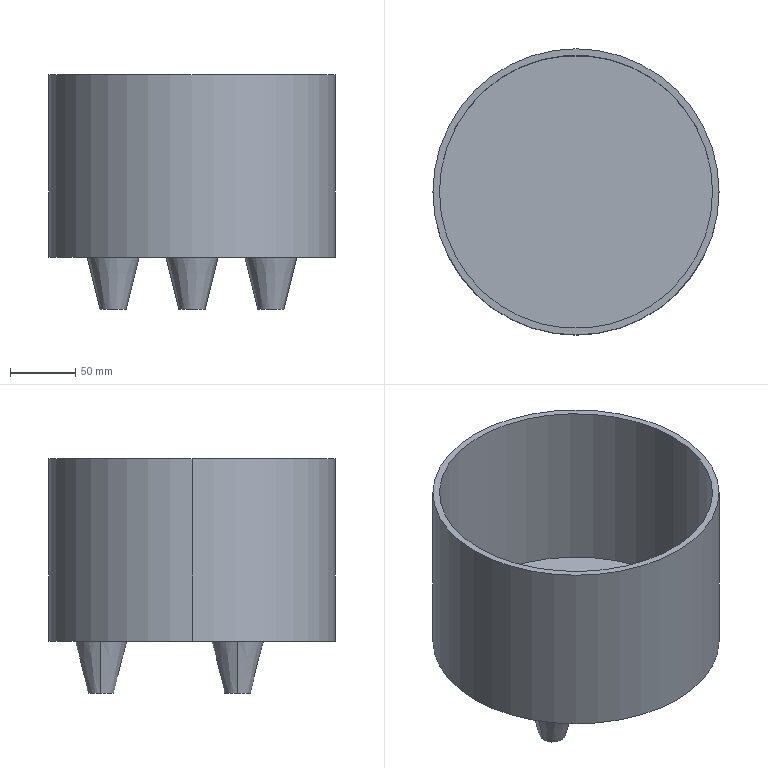Part | STEP file | 333_4 | 1 solid | 16 faces | box 220 x 220 x 180 mm | volume 733955 mm3 | cone 6 | plane 6 | cylinder 4 | commonest cylinder face diameters 210 x2 220 x2
STEP:
#1=CARTESIAN_POINT('',(0.,0.,0.));
#2=DIRECTION('',(0.,0.,1.));
#3=DIRECTION('',(1.,0.,0.));
#4=AXIS2_PLACEMENT_3D('',#1,#2,#3);
#5=CARTESIAN_POINT('',(-110.,0.,40.));
#6=VERTEX_POINT('',#5);
#7=CARTESIAN_POINT('',(110.,0.,40.));
#8=VERTEX_POINT('',#7);
#9=CARTESIAN_POINT('',(0.,0.,40.));
#10=DIRECTION('',(0.,0.,-1.));
#11=DIRECTION('',(-1.,0.,0.));
#12=AXIS2_PLACEMENT_3D('',#9,#10,#11);
#13=CIRCLE('',#12,110.);
#14=CARTESIAN_POINT('',(0.,0.,-30.));
#15=DIRECTION('',(0.,0.,-1.));
#16=DIRECTION('',(-1.,0.,0.));
#17=AXIS2_PLACEMENT_3D('',#14,#15,#16);
#18=CYLINDRICAL_SURFACE('',#17,110.);
#19=CARTESIAN_POINT('',(0.,-70.));
#20=DIRECTION('',(1.,0.));
#21=VECTOR('',#20,1.);
#22=LINE('',#19,#21);
#23=(GEOMETRIC_REPRESENTATION_CONTEXT(2)PARAMETRIC_REPRESENTATION_CONTEXT()REPRESENTATION_CONTEXT('',''));
#24=DEFINITIONAL_REPRESENTATION('',(#22),#23);
#25=PCURVE('',#18,#24);
#26=CARTESIAN_POINT('',(0.,0.,40.));
#27=DIRECTION('',(0.,0.,-1.));
#28=DIRECTION('',(-1.,0.,0.));
#29=AXIS2_PLACEMENT_3D('',#26,#27,#28);
#30=PLANE('',#29);
#31=CARTESIAN_POINT('',(0.,0.));
#32=DIRECTION('',(1.,0.));
#33=AXIS2_PLACEMENT_2D('',#31,#32);
#34=CIRCLE('',#33,110.);
#35=(GEOMETRIC_REPRESENTATION_CONTEXT(2)PARAMETRIC_REPRESENTATION_CONTEXT()REPRESENTATION_CONTEXT('',''));
#36=DEFINITIONAL_REPRESENTATION('',(#34),#35);
#37=PCURVE('',#30,#36);
#38=SURFACE_CURVE('',#13,(#25,#37),.PCURVE_S1.);
#39=EDGE_CURVE('',#6,#8,#38,.T.);
#40=ORIENTED_EDGE('',*,*,#39,.T.);
#41=CARTESIAN_POINT('',(110.,0.,-100.));
#42=VERTEX_POINT('',#41);
#43=CARTESIAN_POINT('',(110.,0.,-30.));
#44=DIRECTION('',(0.,0.,-1.));
#45=VECTOR('',#44,1.);
#46=LINE('',#43,#45);
#47=CARTESIAN_POINT('',(3.142,0.));
#48=DIRECTION('',(0.,1.));
#49=VECTOR('',#48,1.);
#50=LINE('',#47,#49);
#51=(GEOMETRIC_REPRESENTATION_CONTEXT(2)PARAMETRIC_REPRESENTATION_CONTEXT()REPRESENTATION_CONTEXT('',''));
#52=DEFINITIONAL_REPRESENTATION('',(#50),#51);
#53=PCURVE('',#18,#52);
#54=CARTESIAN_POINT('',(0.,0.,-30.));
#55=DIRECTION('',(0.,0.,-1.));
#56=DIRECTION('',(-1.,0.,0.));
#57=AXIS2_PLACEMENT_3D('',#54,#55,#56);
#58=CYLINDRICAL_SURFACE('',#57,110.);
#59=CARTESIAN_POINT('',(3.142,0.));
#60=DIRECTION('',(0.,1.));
#61=VECTOR('',#60,1.);
#62=LINE('',#59,#61);
#63=(GEOMETRIC_REPRESENTATION_CONTEXT(2)PARAMETRIC_REPRESENTATION_CONTEXT()REPRESENTATION_CONTEXT('',''));
#64=DEFINITIONAL_REPRESENTATION('',(#62),#63);
#65=PCURVE('',#58,#64);
#66=SURFACE_CURVE('',#46,(#53,#65),.PCURVE_S1.);
#67=EDGE_CURVE('',#8,#42,#66,.T.);
#68=ORIENTED_EDGE('',*,*,#67,.T.);
#69=CARTESIAN_POINT('',(-110.,0.,-100.));
#70=VERTEX_POINT('',#69);
#71=CARTESIAN_POINT('',(0.,0.,-100.));
#72=DIRECTION('',(0.,0.,1.));
#73=DIRECTION('',(-1.,0.,0.));
#74=AXIS2_PLACEMENT_3D('',#71,#72,#73);
#75=CIRCLE('',#74,110.);
#76=CARTESIAN_POINT('',(6.283,70.));
#77=DIRECTION('',(-1.,0.));
#78=VECTOR('',#77,1.);
#79=LINE('',#76,#78);
#80=(GEOMETRIC_REPRESENTATION_CONTEXT(2)PARAMETRIC_REPRESENTATION_CONTEXT()REPRESENTATION_CONTEXT('',''));
#81=DEFINITIONAL_REPRESENTATION('',(#79),#80);
#82=PCURVE('',#18,#81);
#83=CARTESIAN_POINT('',(-110.,0.,-100.));
#84=DIRECTION('',(0.,0.,-1.));
#85=DIRECTION('',(-1.,0.,0.));
#86=AXIS2_PLACEMENT_3D('',#83,#84,#85);
#87=PLANE('',#86);
#88=CARTESIAN_POINT('',(0.,0.));
#89=CARTESIAN_POINT('',(0.,-190.526));
#90=CARTESIAN_POINT('',(-165.,-95.263));
#91=CARTESIAN_POINT('',(-330.,0.));
#92=CARTESIAN_POINT('',(-165.,95.263));
#93=CARTESIAN_POINT('',(0.,190.526));
#94=CARTESIAN_POINT('',(0.,0.));
#95=(BOUNDED_CURVE()B_SPLINE_CURVE(2,(#88,#89,#90,#91,#92,#93,#94),.UNSPECIFIED.,.T.,.F.)B_SPLINE_CURVE_WITH_KNOTS((1,2,2,2,2,1),(-2.094,0.,2.094,4.189,6.283,8.378),.UNSPECIFIED.)CURVE()GEOMETRIC_REPRESENTATION_ITEM()RATIONAL_B_SPLINE_CURVE((1.,0.5,1.,0.5,1.,0.5,1.))REPRESENTATION_ITEM(''));
#96=(GEOMETRIC_REPRESENTATION_CONTEXT(2)PARAMETRIC_REPRESENTATION_CONTEXT()REPRESENTATION_CONTEXT('',''));
#97=DEFINITIONAL_REPRESENTATION('',(#95),#96);
#98=PCURVE('',#87,#97);
#99=SURFACE_CURVE('',#75,(#82,#98),.PCURVE_S1.);
#100=EDGE_CURVE('',#42,#70,#99,.T.);
#101=ORIENTED_EDGE('',*,*,#100,.T.);
#102=CARTESIAN_POINT('',(-110.,0.,-30.));
#103=DIRECTION('',(0.,0.,-1.));
#104=VECTOR('',#103,1.);
#105=LINE('',#102,#104);
#106=CARTESIAN_POINT('',(0.,0.));
#107=DIRECTION('',(0.,1.));
#108=VECTOR('',#107,1.);
#109=LINE('',#106,#108);
#110=(GEOMETRIC_REPRESENTATION_CONTEXT(2)PARAMETRIC_REPRESENTATION_CONTEXT()REPRESENTATION_CONTEXT('',''));
#111=DEFINITIONAL_REPRESENTATION('',(#109),#110);
#112=PCURVE('',#18,#111);
#113=CARTESIAN_POINT('',(6.283,0.));
#114=DIRECTION('',(0.,1.));
#115=VECTOR('',#114,1.);
#116=LINE('',#113,#115);
#117=(GEOMETRIC_REPRESENTATION_CONTEXT(2)PARAMETRIC_REPRESENTATION_CONTEXT()REPRESENTATION_CONTEXT('',''));
#118=DEFINITIONAL_REPRESENTATION('',(#116),#117);
#119=PCURVE('',#58,#118);
#120=SURFACE_CURVE('',#105,(#112,#119),.PCURVE_S1.);
#121=EDGE_CURVE('',#6,#70,#120,.T.);
#122=ORIENTED_EDGE('',*,*,#121,.F.);
#123=EDGE_LOOP('',(#40,#68,#101,#122));
#124=FACE_BOUND('',#123,.T.);
#125=ADVANCED_FACE('',(#124),#18,.T.);
#126=CARTESIAN_POINT('',(-105.,0.,40.));
#127=VERTEX_POINT('',#126);
#128=CARTESIAN_POINT('',(-105.,0.,-95.));
#129=VERTEX_POINT('',#128);
#130=CARTESIAN_POINT('',(-105.,0.,-30.));
#131=DIRECTION('',(0.,0.,-1.));
#132=VECTOR('',#131,1.);
#133=LINE('',#130,#132);
#134=CARTESIAN_POINT('',(0.,0.,-30.));
#135=DIRECTION('',(0.,0.,-1.));
#136=DIRECTION('',(-1.,0.,0.));
#137=AXIS2_PLACEMENT_3D('',#134,#135,#136);
#138=CYLINDRICAL_SURFACE('',#137,105.);
#139=CARTESIAN_POINT('',(6.283,0.));
#140=DIRECTION('',(0.,1.));
#141=VECTOR('',#140,1.);
#142=LINE('',#139,#141);
#143=(GEOMETRIC_REPRESENTATION_CONTEXT(2)PARAMETRIC_REPRESENTATION_CONTEXT()REPRESENTATION_CONTEXT('',''));
#144=DEFINITIONAL_REPRESENTATION('',(#142),#143);
#145=PCURVE('',#138,#144);
#146=CARTESIAN_POINT('',(0.,0.,-30.));
#147=DIRECTION('',(0.,0.,-1.));
#148=DIRECTION('',(-1.,0.,0.));
#149=AXIS2_PLACEMENT_3D('',#146,#147,#148);
#150=CYLINDRICAL_SURFACE('',#149,105.);
#151=CARTESIAN_POINT('',(0.,0.));
#152=DIRECTION('',(0.,1.));
#153=VECTOR('',#152,1.);
#154=LINE('',#151,#153);
#155=(GEOMETRIC_REPRESENTATION_CONTEXT(2)PARAMETRIC_REPRESENTATION_CONTEXT()REPRESENTATION_CONTEXT('',''));
#156=DEFINITIONAL_REPRESENTATION('',(#154),#155);
#157=PCURVE('',#150,#156);
#158=SURFACE_CURVE('',#133,(#145,#157),.PCURVE_S1.);
#159=EDGE_CURVE('',#127,#129,#158,.T.);
#160=ORIENTED_EDGE('',*,*,#159,.T.);
#161=CARTESIAN_POINT('',(105.,0.,-95.));
#162=VERTEX_POINT('',#161);
#163=CARTESIAN_POINT('',(0.,0.,-95.));
#164=DIRECTION('',(0.,0.,1.));
#165=DIRECTION('',(-1.,0.,0.));
#166=AXIS2_PLACEMENT_3D('',#163,#164,#165);
#167=CIRCLE('',#166,105.);
#168=CARTESIAN_POINT('',(6.283,65.));
#169=DIRECTION('',(-1.,0.));
#170=VECTOR('',#169,1.);
#171=LINE('',#168,#170);
#172=(GEOMETRIC_REPRESENTATION_CONTEXT(2)PARAMETRIC_REPRESENTATION_CONTEXT()REPRESENTATION_CONTEXT('',''));
#173=DEFINITIONAL_REPRESENTATION('',(#171),#172);
#174=PCURVE('',#138,#173);
#175=CARTESIAN_POINT('',(-110.,0.,-95.));
#176=DIRECTION('',(0.,0.,-1.));
#177=DIRECTION('',(-1.,0.,0.));
#178=AXIS2_PLACEMENT_3D('',#175,#176,#177);
#179=PLANE('',#178);
#180=CARTESIAN_POINT('',(-5.,0.));
#181=CARTESIAN_POINT('',(-5.,-181.865));
#182=CARTESIAN_POINT('',(-162.5,-90.933));
#183=CARTESIAN_POINT('',(-320.,0.));
#184=CARTESIAN_POINT('',(-162.5,90.933));
#185=CARTESIAN_POINT('',(-5.,181.865));
#186=CARTESIAN_POINT('',(-5.,0.));
#187=(BOUNDED_CURVE()B_SPLINE_CURVE(2,(#180,#181,#182,#183,#184,#185,#186),.UNSPECIFIED.,.T.,.F.)B_SPLINE_CURVE_WITH_KNOTS((1,2,2,2,2,1),(-2.094,0.,2.094,4.189,6.283,8.378),.UNSPECIFIED.)CURVE()GEOMETRIC_REPRESENTATION_ITEM()RATIONAL_B_SPLINE_CURVE((1.,0.5,1.,0.5,1.,0.5,1.))REPRESENTATION_ITEM(''));
#188=(GEOMETRIC_REPRESENTATION_CONTEXT(2)PARAMETRIC_REPRESENTATION_CONTEXT()REPRESENTATION_CONTEXT('',''));
#189=DEFINITIONAL_REPRESENTATION('',(#187),#188);
#190=PCURVE('',#179,#189);
#191=SURFACE_CURVE('',#167,(#174,#190),.PCURVE_S1.);
#192=EDGE_CURVE('',#129,#162,#191,.T.);
#193=ORIENTED_EDGE('',*,*,#192,.T.);
#194=CARTESIAN_POINT('',(105.,0.,40.));
#195=VERTEX_POINT('',#194);
#196=CARTESIAN_POINT('',(105.,0.,-30.));
#197=DIRECTION('',(0.,0.,-1.));
#198=VECTOR('',#197,1.);
#199=LINE('',#196,#198);
#200=CARTESIAN_POINT('',(3.142,0.));
#201=DIRECTION('',(0.,1.));
#202=VECTOR('',#201,1.);
#203=LINE('',#200,#202);
#204=(GEOMETRIC_REPRESENTATION_CONTEXT(2)PARAMETRIC_REPRESENTATION_CONTEXT()REPRESENTATION_CONTEXT('',''));
#205=DEFINITIONAL_REPRESENTATION('',(#203),#204);
#206=PCURVE('',#138,#205);
#207=CARTESIAN_POINT('',(3.142,0.));
#208=DIRECTION('',(0.,1.));
#209=VECTOR('',#208,1.);
#210=LINE('',#207,#209);
#211=(GEOMETRIC_REPRESENTATION_CONTEXT(2)PARAMETRIC_REPRESENTATION_CONTEXT()REPRESENTATION_CONTEXT('',''));
#212=DEFINITIONAL_REPRESENTATION('',(#210),#211);
#213=PCURVE('',#150,#212);
#214=SURFACE_CURVE('',#199,(#206,#213),.PCURVE_S1.);
#215=EDGE_CURVE('',#195,#162,#214,.T.);
#216=ORIENTED_EDGE('',*,*,#215,.F.);
#217=CARTESIAN_POINT('',(0.,0.,40.));
#218=DIRECTION('',(0.,0.,1.));
#219=DIRECTION('',(-1.,0.,0.));
#220=AXIS2_PLACEMENT_3D('',#217,#218,#219);
#221=CIRCLE('',#220,105.);
#222=CARTESIAN_POINT('',(6.283,-70.));
#223=DIRECTION('',(-1.,0.));
#224=VECTOR('',#223,1.);
#225=LINE('',#222,#224);
#226=(GEOMETRIC_REPRESENTATION_CONTEXT(2)PARAMETRIC_REPRESENTATION_CONTEXT()REPRESENTATION_CONTEXT('',''));
#227=DEFINITIONAL_REPRESENTATION('',(#225),#226);
#228=PCURVE('',#138,#227);
#229=CARTESIAN_POINT('',(105.,0.));
#230=CARTESIAN_POINT('',(105.,-181.865));
#231=CARTESIAN_POINT('',(-52.5,-90.933));
#232=CARTESIAN_POINT('',(-210.,0.));
#233=CARTESIAN_POINT('',(-52.5,90.933));
#234=CARTESIAN_POINT('',(105.,181.865));
#235=CARTESIAN_POINT('',(105.,0.));
#236=(BOUNDED_CURVE()B_SPLINE_CURVE(2,(#229,#230,#231,#232,#233,#234,#235),.UNSPECIFIED.,.T.,.F.)B_SPLINE_CURVE_WITH_KNOTS((1,2,2,2,2,1),(-2.094,0.,2.094,4.189,6.283,8.378),.UNSPECIFIED.)CURVE()GEOMETRIC_REPRESENTATION_ITEM()RATIONAL_B_SPLINE_CURVE((1.,0.5,1.,0.5,1.,0.5,1.))REPRESENTATION_ITEM(''));
#237=(GEOMETRIC_REPRESENTATION_CONTEXT(2)PARAMETRIC_REPRESENTATION_CONTEXT()REPRESENTATION_CONTEXT('',''));
#238=DEFINITIONAL_REPRESENTATION('',(#236),#237);
#239=PCURVE('',#30,#238);
#240=SURFACE_CURVE('',#221,(#228,#239),.PCURVE_S1.);
#241=EDGE_CURVE('',#127,#195,#240,.T.);
#242=ORIENTED_EDGE('',*,*,#241,.F.);
#243=EDGE_LOOP('',(#160,#193,#216,#242));
#244=FACE_BOUND('',#243,.F.);
#245=ADVANCED_FACE('',(#244),#138,.F.);
#246=CARTESIAN_POINT('',(70.622,-35.,-140.));
#247=VERTEX_POINT('',#246);
#248=CARTESIAN_POINT('',(50.622,-35.,-140.));
#249=VERTEX_POINT('',#248);
#250=CARTESIAN_POINT('',(60.622,-35.,-140.));
#251=DIRECTION('',(0.,0.,1.));
#252=DIRECTION('',(1.,0.,0.));
#253=AXIS2_PLACEMENT_3D('',#250,#251,#252);
#254=CIRCLE('',#253,10.);
#255=CARTESIAN_POINT('',(60.622,-35.,-100.));
#256=DIRECTION('',(0.,0.,1.));
#257=DIRECTION('',(1.,0.,0.));
#258=AXIS2_PLACEMENT_3D('',#255,#256,#257);
#259=CONICAL_SURFACE('',#258,20.,0.245);
#260=CARTESIAN_POINT('',(0.,-40.));
#261=DIRECTION('',(1.,0.));
#262=VECTOR('',#261,1.);
#263=LINE('',#260,#262);
#264=(GEOMETRIC_REPRESENTATION_CONTEXT(2)PARAMETRIC_REPRESENTATION_CONTEXT()REPRESENTATION_CONTEXT('',''));
#265=DEFINITIONAL_REPRESENTATION('',(#263),#264);
#266=PCURVE('',#259,#265);
#267=CARTESIAN_POINT('',(0.,80.,-140.));
#268=DIRECTION('',(0.,0.,-1.));
#269=DIRECTION('',(-1.,0.,0.));
#270=AXIS2_PLACEMENT_3D('',#267,#268,#269);
#271=PLANE('',#270);
#272=CARTESIAN_POINT('',(-70.622,-115.));
#273=CARTESIAN_POINT('',(-70.622,-97.679));
#274=CARTESIAN_POINT('',(-55.622,-106.34));
#275=CARTESIAN_POINT('',(-40.622,-115.));
#276=CARTESIAN_POINT('',(-55.622,-123.66));
#277=CARTESIAN_POINT('',(-70.622,-132.321));
#278=CARTESIAN_POINT('',(-70.622,-115.));
#279=(BOUNDED_CURVE()B_SPLINE_CURVE(2,(#272,#273,#274,#275,#276,#277,#278),.UNSPECIFIED.,.T.,.F.)B_SPLINE_CURVE_WITH_KNOTS((1,2,2,2,2,1),(-2.094,0.,2.094,4.189,6.283,8.378),.UNSPECIFIED.)CURVE()GEOMETRIC_REPRESENTATION_ITEM()RATIONAL_B_SPLINE_CURVE((1.,0.5,1.,0.5,1.,0.5,1.))REPRESENTATION_ITEM(''));
#280=(GEOMETRIC_REPRESENTATION_CONTEXT(2)PARAMETRIC_REPRESENTATION_CONTEXT()REPRESENTATION_CONTEXT('',''));
#281=DEFINITIONAL_REPRESENTATION('',(#279),#280);
#282=PCURVE('',#271,#281);
#283=SURFACE_CURVE('',#254,(#266,#282),.PCURVE_S1.);
#284=EDGE_CURVE('',#247,#249,#283,.T.);
#285=ORIENTED_EDGE('',*,*,#284,.T.);
#286=CARTESIAN_POINT('',(40.622,-35.,-100.));
#287=VERTEX_POINT('',#286);
#288=CARTESIAN_POINT('',(40.622,-35.,-100.));
#289=DIRECTION('',(-0.2425,0.,0.9701));
#290=VECTOR('',#289,1.);
#291=LINE('',#288,#290);
#292=CARTESIAN_POINT('',(3.142,0.));
#293=DIRECTION('',(0.,1.));
#294=VECTOR('',#293,1.);
#295=LINE('',#292,#294);
#296=(GEOMETRIC_REPRESENTATION_CONTEXT(2)PARAMETRIC_REPRESENTATION_CONTEXT()REPRESENTATION_CONTEXT('',''));
#297=DEFINITIONAL_REPRESENTATION('',(#295),#296);
#298=PCURVE('',#259,#297);
#299=CARTESIAN_POINT('',(60.622,-35.,-100.));
#300=DIRECTION('',(0.,0.,1.));
#301=DIRECTION('',(1.,0.,0.));
#302=AXIS2_PLACEMENT_3D('',#299,#300,#301);
#303=CONICAL_SURFACE('',#302,20.,0.245);
#304=CARTESIAN_POINT('',(3.142,0.));
#305=DIRECTION('',(0.,1.));
#306=VECTOR('',#305,1.);
#307=LINE('',#304,#306);
#308=(GEOMETRIC_REPRESENTATION_CONTEXT(2)PARAMETRIC_REPRESENTATION_CONTEXT()REPRESENTATION_CONTEXT('',''));
#309=DEFINITIONAL_REPRESENTATION('',(#307),#308);
#310=PCURVE('',#303,#309);
#311=SURFACE_CURVE('',#291,(#298,#310),.PCURVE_S1.);
#312=EDGE_CURVE('',#249,#287,#311,.T.);
#313=ORIENTED_EDGE('',*,*,#312,.T.);
#314=CARTESIAN_POINT('',(80.622,-35.,-100.));
#315=VERTEX_POINT('',#314);
#316=CARTESIAN_POINT('',(60.622,-35.,-100.));
#317=DIRECTION('',(0.,0.,1.));
#318=DIRECTION('',(1.,0.,0.));
#319=AXIS2_PLACEMENT_3D('',#316,#317,#318);
#320=CIRCLE('',#319,20.);
#321=CARTESIAN_POINT('',(0.,0.));
#322=DIRECTION('',(1.,0.));
#323=VECTOR('',#322,1.);
#324=LINE('',#321,#323);
#325=(GEOMETRIC_REPRESENTATION_CONTEXT(2)PARAMETRIC_REPRESENTATION_CONTEXT()REPRESENTATION_CONTEXT('',''));
#326=DEFINITIONAL_REPRESENTATION('',(#324),#325);
#327=PCURVE('',#259,#326);
#328=CARTESIAN_POINT('',(-190.622,-35.));
#329=CARTESIAN_POINT('',(-190.622,-0.359));
#330=CARTESIAN_POINT('',(-160.622,-17.679));
#331=CARTESIAN_POINT('',(-130.622,-35.));
#332=CARTESIAN_POINT('',(-160.622,-52.321));
#333=CARTESIAN_POINT('',(-190.622,-69.641));
#334=CARTESIAN_POINT('',(-190.622,-35.));
#335=(BOUNDED_CURVE()B_SPLINE_CURVE(2,(#328,#329,#330,#331,#332,#333,#334),.UNSPECIFIED.,.T.,.F.)B_SPLINE_CURVE_WITH_KNOTS((1,2,2,2,2,1),(-2.094,0.,2.094,4.189,6.283,8.378),.UNSPECIFIED.)CURVE()GEOMETRIC_REPRESENTATION_ITEM()RATIONAL_B_SPLINE_CURVE((1.,0.5,1.,0.5,1.,0.5,1.))REPRESENTATION_ITEM(''));
#336=(GEOMETRIC_REPRESENTATION_CONTEXT(2)PARAMETRIC_REPRESENTATION_CONTEXT()REPRESENTATION_CONTEXT('',''));
#337=DEFINITIONAL_REPRESENTATION('',(#335),#336);
#338=PCURVE('',#87,#337);
#339=SURFACE_CURVE('',#320,(#327,#338),.PCURVE_S1.);
#340=EDGE_CURVE('',#315,#287,#339,.T.);
#341=ORIENTED_EDGE('',*,*,#340,.F.);
#342=CARTESIAN_POINT('',(80.622,-35.,-100.));
#343=DIRECTION('',(0.2425,0.,0.9701));
#344=VECTOR('',#343,1.);
#345=LINE('',#342,#344);
#346=CARTESIAN_POINT('',(0.,0.));
#347=DIRECTION('',(0.,1.));
#348=VECTOR('',#347,1.);
#349=LINE('',#346,#348);
#350=(GEOMETRIC_REPRESENTATION_CONTEXT(2)PARAMETRIC_REPRESENTATION_CONTEXT()REPRESENTATION_CONTEXT('',''));
#351=DEFINITIONAL_REPRESENTATION('',(#349),#350);
#352=PCURVE('',#259,#351);
#353=CARTESIAN_POINT('',(6.283,0.));
#354=DIRECTION('',(0.,1.));
#355=VECTOR('',#354,1.);
#356=LINE('',#353,#355);
#357=(GEOMETRIC_REPRESENTATION_CONTEXT(2)PARAMETRIC_REPRESENTATION_CONTEXT()REPRESENTATION_CONTEXT('',''));
#358=DEFINITIONAL_REPRESENTATION('',(#356),#357);
#359=PCURVE('',#303,#358);
#360=SURFACE_CURVE('',#345,(#352,#359),.PCURVE_S1.);
#361=EDGE_CURVE('',#247,#315,#360,.T.);
#362=ORIENTED_EDGE('',*,*,#361,.F.);
#363=EDGE_LOOP('',(#285,#313,#341,#362));
#364=FACE_BOUND('',#363,.T.);
#365=ADVANCED_FACE('',(#364),#259,.T.);
#366=CARTESIAN_POINT('',(-50.622,-35.,-140.));
#367=VERTEX_POINT('',#366);
#368=CARTESIAN_POINT('',(-70.622,-35.,-140.));
#369=VERTEX_POINT('',#368);
#370=CARTESIAN_POINT('',(-60.622,-35.,-140.));
#371=DIRECTION('',(0.,0.,1.));
#372=DIRECTION('',(1.,0.,0.));
#373=AXIS2_PLACEMENT_3D('',#370,#371,#372);
#374=CIRCLE('',#373,10.);
#375=CARTESIAN_POINT('',(-60.622,-35.,-100.));
#376=DIRECTION('',(0.,0.,1.));
#377=DIRECTION('',(1.,0.,0.));
#378=AXIS2_PLACEMENT_3D('',#375,#376,#377);
#379=CONICAL_SURFACE('',#378,20.,0.245);
#380=CARTESIAN_POINT('',(0.,-40.));
#381=DIRECTION('',(1.,0.));
#382=VECTOR('',#381,1.);
#383=LINE('',#380,#382);
#384=(GEOMETRIC_REPRESENTATION_CONTEXT(2)PARAMETRIC_REPRESENTATION_CONTEXT()REPRESENTATION_CONTEXT('',''));
#385=DEFINITIONAL_REPRESENTATION('',(#383),#384);
#386=PCURVE('',#379,#385);
#387=CARTESIAN_POINT('',(0.,80.,-140.));
#388=DIRECTION('',(0.,0.,-1.));
#389=DIRECTION('',(-1.,0.,0.));
#390=AXIS2_PLACEMENT_3D('',#387,#388,#389);
#391=PLANE('',#390);
#392=CARTESIAN_POINT('',(50.622,-115.));
#393=CARTESIAN_POINT('',(50.622,-97.679));
#394=CARTESIAN_POINT('',(65.622,-106.34));
#395=CARTESIAN_POINT('',(80.622,-115.));
#396=CARTESIAN_POINT('',(65.622,-123.66));
#397=CARTESIAN_POINT('',(50.622,-132.321));
#398=CARTESIAN_POINT('',(50.622,-115.));
#399=(BOUNDED_CURVE()B_SPLINE_CURVE(2,(#392,#393,#394,#395,#396,#397,#398),.UNSPECIFIED.,.T.,.F.)B_SPLINE_CURVE_WITH_KNOTS((1,2,2,2,2,1),(-2.094,0.,2.094,4.189,6.283,8.378),.UNSPECIFIED.)CURVE()GEOMETRIC_REPRESENTATION_ITEM()RATIONAL_B_SPLINE_CURVE((1.,0.5,1.,0.5,1.,0.5,1.))REPRESENTATION_ITEM(''));
#400=(GEOMETRIC_REPRESENTATION_CONTEXT(2)PARAMETRIC_REPRESENTATION_CONTEXT()REPRESENTATION_CONTEXT('',''));
#401=DEFINITIONAL_REPRESENTATION('',(#399),#400);
#402=PCURVE('',#391,#401);
#403=SURFACE_CURVE('',#374,(#386,#402),.PCURVE_S1.);
#404=EDGE_CURVE('',#367,#369,#403,.T.);
#405=ORIENTED_EDGE('',*,*,#404,.T.);
#406=CARTESIAN_POINT('',(-80.622,-35.,-100.));
#407=VERTEX_POINT('',#406);
#408=CARTESIAN_POINT('',(-80.622,-35.,-100.));
#409=DIRECTION('',(-0.2425,0.,0.9701));
#410=VECTOR('',#409,1.);
#411=LINE('',#408,#410);
#412=CARTESIAN_POINT('',(3.142,0.));
#413=DIRECTION('',(0.,1.));
#414=VECTOR('',#413,1.);
#415=LINE('',#412,#414);
#416=(GEOMETRIC_REPRESENTATION_CONTEXT(2)PARAMETRIC_REPRESENTATION_CONTEXT()REPRESENTATION_CONTEXT('',''));
#417=DEFINITIONAL_REPRESENTATION('',(#415),#416);
#418=PCURVE('',#379,#417);
#419=CARTESIAN_POINT('',(-60.622,-35.,-100.));
#420=DIRECTION('',(0.,0.,1.));
#421=DIRECTION('',(1.,0.,0.));
#422=AXIS2_PLACEMENT_3D('',#419,#420,#421);
#423=CONICAL_SURFACE('',#422,20.,0.245);
#424=CARTESIAN_POINT('',(3.142,0.));
#425=DIRECTION('',(0.,1.));
#426=VECTOR('',#425,1.);
#427=LINE('',#424,#426);
#428=(GEOMETRIC_REPRESENTATION_CONTEXT(2)PARAMETRIC_REPRESENTATION_CONTEXT()REPRESENTATION_CONTEXT('',''));
#429=DEFINITIONAL_REPRESENTATION('',(#427),#428);
#430=PCURVE('',#423,#429);
#431=SURFACE_CURVE('',#411,(#418,#430),.PCURVE_S1.);
#432=EDGE_CURVE('',#369,#407,#431,.T.);
#433=ORIENTED_EDGE('',*,*,#432,.T.);
#434=CARTESIAN_POINT('',(-40.622,-35.,-100.));
#435=VERTEX_POINT('',#434);
#436=CARTESIAN_POINT('',(-60.622,-35.,-100.));
#437=DIRECTION('',(0.,0.,1.));
#438=DIRECTION('',(1.,0.,0.));
#439=AXIS2_PLACEMENT_3D('',#436,#437,#438);
#440=CIRCLE('',#439,20.);
#441=CARTESIAN_POINT('',(0.,0.));
#442=DIRECTION('',(1.,0.));
#443=VECTOR('',#442,1.);
#444=LINE('',#441,#443);
#445=(GEOMETRIC_REPRESENTATION_CONTEXT(2)PARAMETRIC_REPRESENTATION_CONTEXT()REPRESENTATION_CONTEXT('',''));
#446=DEFINITIONAL_REPRESENTATION('',(#444),#445);
#447=PCURVE('',#379,#446);
#448=CARTESIAN_POINT('',(-69.378,-35.));
#449=CARTESIAN_POINT('',(-69.378,-0.359));
#450=CARTESIAN_POINT('',(-39.378,-17.679));
#451=CARTESIAN_POINT('',(-9.378,-35.));
#452=CARTESIAN_POINT('',(-39.378,-52.321));
#453=CARTESIAN_POINT('',(-69.378,-69.641));
#454=CARTESIAN_POINT('',(-69.378,-35.));
#455=(BOUNDED_CURVE()B_SPLINE_CURVE(2,(#448,#449,#450,#451,#452,#453,#454),.UNSPECIFIED.,.T.,.F.)B_SPLINE_CURVE_WITH_KNOTS((1,2,2,2,2,1),(-2.094,0.,2.094,4.189,6.283,8.378),.UNSPECIFIED.)CURVE()GEOMETRIC_REPRESENTATION_ITEM()RATIONAL_B_SPLINE_CURVE((1.,0.5,1.,0.5,1.,0.5,1.))REPRESENTATION_ITEM(''));
#456=(GEOMETRIC_REPRESENTATION_CONTEXT(2)PARAMETRIC_REPRESENTATION_CONTEXT()REPRESENTATION_CONTEXT('',''));
#457=DEFINITIONAL_REPRESENTATION('',(#455),#456);
#458=PCURVE('',#87,#457);
#459=SURFACE_CURVE('',#440,(#447,#458),.PCURVE_S1.);
#460=EDGE_CURVE('',#435,#407,#459,.T.);
#461=ORIENTED_EDGE('',*,*,#460,.F.);
#462=CARTESIAN_POINT('',(-40.622,-35.,-100.));
#463=DIRECTION('',(0.2425,0.,0.9701));
#464=VECTOR('',#463,1.);
#465=LINE('',#462,#464);
#466=CARTESIAN_POINT('',(0.,0.));
#467=DIRECTION('',(0.,1.));
#468=VECTOR('',#467,1.);
#469=LINE('',#466,#468);
#470=(GEOMETRIC_REPRESENTATION_CONTEXT(2)PARAMETRIC_REPRESENTATION_CONTEXT()REPRESENTATION_CONTEXT('',''));
#471=DEFINITIONAL_REPRESENTATION('',(#469),#470);
#472=PCURVE('',#379,#471);
#473=CARTESIAN_POINT('',(6.283,0.));
#474=DIRECTION('',(0.,1.));
#475=VECTOR('',#474,1.);
#476=LINE('',#473,#475);
#477=(GEOMETRIC_REPRESENTATION_CONTEXT(2)PARAMETRIC_REPRESENTATION_CONTEXT()REPRESENTATION_CONTEXT('',''));
#478=DEFINITIONAL_REPRESENTATION('',(#476),#477);
#479=PCURVE('',#423,#478);
#480=SURFACE_CURVE('',#465,(#472,#479),.PCURVE_S1.);
#481=EDGE_CURVE('',#367,#435,#480,.T.);
#482=ORIENTED_EDGE('',*,*,#481,.F.);
#483=EDGE_LOOP('',(#405,#433,#461,#482));
#484=FACE_BOUND('',#483,.T.);
#485=ADVANCED_FACE('',(#484),#379,.T.);
#486=CARTESIAN_POINT('',(10.,70.,-140.));
#487=VERTEX_POINT('',#486);
#488=CARTESIAN_POINT('',(-10.,70.,-140.));
#489=VERTEX_POINT('',#488);
#490=CARTESIAN_POINT('',(0.,70.,-140.));
#491=DIRECTION('',(0.,0.,1.));
#492=DIRECTION('',(1.,0.,0.));
#493=AXIS2_PLACEMENT_3D('',#490,#491,#492);
#494=CIRCLE('',#493,10.);
#495=CARTESIAN_POINT('',(0.,70.,-100.));
#496=DIRECTION('',(0.,0.,1.));
#497=DIRECTION('',(1.,0.,0.));
#498=AXIS2_PLACEMENT_3D('',#495,#496,#497);
#499=CONICAL_SURFACE('',#498,20.,0.245);
#500=CARTESIAN_POINT('',(0.,-40.));
#501=DIRECTION('',(1.,0.));
#502=VECTOR('',#501,1.);
#503=LINE('',#500,#502);
#504=(GEOMETRIC_REPRESENTATION_CONTEXT(2)PARAMETRIC_REPRESENTATION_CONTEXT()REPRESENTATION_CONTEXT('',''));
#505=DEFINITIONAL_REPRESENTATION('',(#503),#504);
#506=PCURVE('',#499,#505);
#507=CARTESIAN_POINT('',(0.,80.,-140.));
#508=DIRECTION('',(0.,0.,-1.));
#509=DIRECTION('',(-1.,0.,0.));
#510=AXIS2_PLACEMENT_3D('',#507,#508,#509);
#511=PLANE('',#510);
#512=CARTESIAN_POINT('',(-10.,-10.));
#513=CARTESIAN_POINT('',(-10.,7.321));
#514=CARTESIAN_POINT('',(5.,-1.34));
#515=CARTESIAN_POINT('',(20.,-10.));
#516=CARTESIAN_POINT('',(5.,-18.66));
#517=CARTESIAN_POINT('',(-10.,-27.321));
#518=CARTESIAN_POINT('',(-10.,-10.));
#519=(BOUNDED_CURVE()B_SPLINE_CURVE(2,(#512,#513,#514,#515,#516,#517,#518),.UNSPECIFIED.,.T.,.F.)B_SPLINE_CURVE_WITH_KNOTS((1,2,2,2,2,1),(-2.094,0.,2.094,4.189,6.283,8.378),.UNSPECIFIED.)CURVE()GEOMETRIC_REPRESENTATION_ITEM()RATIONAL_B_SPLINE_CURVE((1.,0.5,1.,0.5,1.,0.5,1.))REPRESENTATION_ITEM(''));
#520=(GEOMETRIC_REPRESENTATION_CONTEXT(2)PARAMETRIC_REPRESENTATION_CONTEXT()REPRESENTATION_CONTEXT('',''));
#521=DEFINITIONAL_REPRESENTATION('',(#519),#520);
#522=PCURVE('',#511,#521);
#523=SURFACE_CURVE('',#494,(#506,#522),.PCURVE_S1.);
#524=EDGE_CURVE('',#487,#489,#523,.T.);
#525=ORIENTED_EDGE('',*,*,#524,.T.);
#526=CARTESIAN_POINT('',(-20.,70.,-100.));
#527=VERTEX_POINT('',#526);
#528=CARTESIAN_POINT('',(-20.,70.,-100.));
#529=DIRECTION('',(-0.2425,0.,0.9701));
#530=VECTOR('',#529,1.);
#531=LINE('',#528,#530);
#532=CARTESIAN_POINT('',(3.142,0.));
#533=DIRECTION('',(0.,1.));
#534=VECTOR('',#533,1.);
#535=LINE('',#532,#534);
#536=(GEOMETRIC_REPRESENTATION_CONTEXT(2)PARAMETRIC_REPRESENTATION_CONTEXT()REPRESENTATION_CONTEXT('',''));
#537=DEFINITIONAL_REPRESENTATION('',(#535),#536);
#538=PCURVE('',#499,#537);
#539=CARTESIAN_POINT('',(0.,70.,-100.));
#540=DIRECTION('',(0.,0.,1.));
#541=DIRECTION('',(1.,0.,0.));
#542=AXIS2_PLACEMENT_3D('',#539,#540,#541);
#543=CONICAL_SURFACE('',#542,20.,0.245);
#544=CARTESIAN_POINT('',(3.142,0.));
#545=DIRECTION('',(0.,1.));
#546=VECTOR('',#545,1.);
#547=LINE('',#544,#546);
#548=(GEOMETRIC_REPRESENTATION_CONTEXT(2)PARAMETRIC_REPRESENTATION_CONTEXT()REPRESENTATION_CONTEXT('',''));
#549=DEFINITIONAL_REPRESENTATION('',(#547),#548);
#550=PCURVE('',#543,#549);
#551=SURFACE_CURVE('',#531,(#538,#550),.PCURVE_S1.);
#552=EDGE_CURVE('',#489,#527,#551,.T.);
#553=ORIENTED_EDGE('',*,*,#552,.T.);
#554=CARTESIAN_POINT('',(20.,70.,-100.));
#555=VERTEX_POINT('',#554);
#556=CARTESIAN_POINT('',(0.,70.,-100.));
#557=DIRECTION('',(0.,0.,1.));
#558=DIRECTION('',(1.,0.,0.));
#559=AXIS2_PLACEMENT_3D('',#556,#557,#558);
#560=CIRCLE('',#559,20.);
#561=CARTESIAN_POINT('',(0.,0.));
#562=DIRECTION('',(1.,0.));
#563=VECTOR('',#562,1.);
#564=LINE('',#561,#563);
#565=(GEOMETRIC_REPRESENTATION_CONTEXT(2)PARAMETRIC_REPRESENTATION_CONTEXT()REPRESENTATION_CONTEXT('',''));
#566=DEFINITIONAL_REPRESENTATION('',(#564),#565);
#567=PCURVE('',#499,#566);
#568=CARTESIAN_POINT('',(-130.,70.));
#569=CARTESIAN_POINT('',(-130.,104.641));
#570=CARTESIAN_POINT('',(-100.,87.321));
#571=CARTESIAN_POINT('',(-70.,70.));
#572=CARTESIAN_POINT('',(-100.,52.679));
#573=CARTESIAN_POINT('',(-130.,35.359));
#574=CARTESIAN_POINT('',(-130.,70.));
#575=(BOUNDED_CURVE()B_SPLINE_CURVE(2,(#568,#569,#570,#571,#572,#573,#574),.UNSPECIFIED.,.T.,.F.)B_SPLINE_CURVE_WITH_KNOTS((1,2,2,2,2,1),(-2.094,0.,2.094,4.189,6.283,8.378),.UNSPECIFIED.)CURVE()GEOMETRIC_REPRESENTATION_ITEM()RATIONAL_B_SPLINE_CURVE((1.,0.5,1.,0.5,1.,0.5,1.))REPRESENTATION_ITEM(''));
#576=(GEOMETRIC_REPRESENTATION_CONTEXT(2)PARAMETRIC_REPRESENTATION_CONTEXT()REPRESENTATION_CONTEXT('',''));
#577=DEFINITIONAL_REPRESENTATION('',(#575),#576);
#578=PCURVE('',#87,#577);
#579=SURFACE_CURVE('',#560,(#567,#578),.PCURVE_S1.);
#580=EDGE_CURVE('',#555,#527,#579,.T.);
#581=ORIENTED_EDGE('',*,*,#580,.F.);
#582=CARTESIAN_POINT('',(20.,70.,-100.));
#583=DIRECTION('',(0.2425,0.,0.9701));
#584=VECTOR('',#583,1.);
#585=LINE('',#582,#584);
#586=CARTESIAN_POINT('',(0.,0.));
#587=DIRECTION('',(0.,1.));
#588=VECTOR('',#587,1.);
#589=LINE('',#586,#588);
#590=(GEOMETRIC_REPRESENTATION_CONTEXT(2)PARAMETRIC_REPRESENTATION_CONTEXT()REPRESENTATION_CONTEXT('',''));
#591=DEFINITIONAL_REPRESENTATION('',(#589),#590);
#592=PCURVE('',#499,#591);
#593=CARTESIAN_POINT('',(6.283,0.));
#594=DIRECTION('',(0.,1.));
#595=VECTOR('',#594,1.);
#596=LINE('',#593,#595);
#597=(GEOMETRIC_REPRESENTATION_CONTEXT(2)PARAMETRIC_REPRESENTATION_CONTEXT()REPRESENTATION_CONTEXT('',''));
#598=DEFINITIONAL_REPRESENTATION('',(#596),#597);
#599=PCURVE('',#543,#598);
#600=SURFACE_CURVE('',#585,(#592,#599),.PCURVE_S1.);
#601=EDGE_CURVE('',#487,#555,#600,.T.);
#602=ORIENTED_EDGE('',*,*,#601,.F.);
#603=EDGE_LOOP('',(#525,#553,#581,#602));
#604=FACE_BOUND('',#603,.T.);
#605=ADVANCED_FACE('',(#604),#499,.T.);
#606=ORIENTED_EDGE('',*,*,#524,.F.);
#607=CARTESIAN_POINT('',(0.,70.,-140.));
#608=DIRECTION('',(0.,0.,1.));
#609=DIRECTION('',(1.,0.,0.));
#610=AXIS2_PLACEMENT_3D('',#607,#608,#609);
#611=CIRCLE('',#610,10.);
#612=CARTESIAN_POINT('',(-10.,-10.));
#613=CARTESIAN_POINT('',(-10.,7.321));
#614=CARTESIAN_POINT('',(5.,-1.34));
#615=CARTESIAN_POINT('',(20.,-10.));
#616=CARTESIAN_POINT('',(5.,-18.66));
#617=CARTESIAN_POINT('',(-10.,-27.321));
#618=CARTESIAN_POINT('',(-10.,-10.));
#619=(BOUNDED_CURVE()B_SPLINE_CURVE(2,(#612,#613,#614,#615,#616,#617,#618),.UNSPECIFIED.,.T.,.F.)B_SPLINE_CURVE_WITH_KNOTS((1,2,2,2,2,1),(-2.094,0.,2.094,4.189,6.283,8.378),.UNSPECIFIED.)CURVE()GEOMETRIC_REPRESENTATION_ITEM()RATIONAL_B_SPLINE_CURVE((1.,0.5,1.,0.5,1.,0.5,1.))REPRESENTATION_ITEM(''));
#620=(GEOMETRIC_REPRESENTATION_CONTEXT(2)PARAMETRIC_REPRESENTATION_CONTEXT()REPRESENTATION_CONTEXT('',''));
#621=DEFINITIONAL_REPRESENTATION('',(#619),#620);
#622=PCURVE('',#511,#621);
#623=CARTESIAN_POINT('',(0.,-40.));
#624=DIRECTION('',(1.,0.));
#625=VECTOR('',#624,1.);
#626=LINE('',#623,#625);
#627=(GEOMETRIC_REPRESENTATION_CONTEXT(2)PARAMETRIC_REPRESENTATION_CONTEXT()REPRESENTATION_CONTEXT('',''));
#628=DEFINITIONAL_REPRESENTATION('',(#626),#627);
#629=PCURVE('',#543,#628);
#630=SURFACE_CURVE('',#611,(#622,#629),.PCURVE_S1.);
#631=EDGE_CURVE('',#489,#487,#630,.T.);
#632=ORIENTED_EDGE('',*,*,#631,.F.);
#633=EDGE_LOOP('',(#606,#632));
#634=FACE_BOUND('',#633,.T.);
#635=ADVANCED_FACE('',(#634),#511,.T.);
#636=ORIENTED_EDGE('',*,*,#404,.F.);
#637=CARTESIAN_POINT('',(-60.622,-35.,-140.));
#638=DIRECTION('',(0.,0.,1.));
#639=DIRECTION('',(1.,0.,0.));
#640=AXIS2_PLACEMENT_3D('',#637,#638,#639);
#641=CIRCLE('',#640,10.);
#642=CARTESIAN_POINT('',(50.622,-115.));
#643=CARTESIAN_POINT('',(50.622,-97.679));
#644=CARTESIAN_POINT('',(65.622,-106.34));
#645=CARTESIAN_POINT('',(80.622,-115.));
#646=CARTESIAN_POINT('',(65.622,-123.66));
#647=CARTESIAN_POINT('',(50.622,-132.321));
#648=CARTESIAN_POINT('',(50.622,-115.));
#649=(BOUNDED_CURVE()B_SPLINE_CURVE(2,(#642,#643,#644,#645,#646,#647,#648),.UNSPECIFIED.,.T.,.F.)B_SPLINE_CURVE_WITH_KNOTS((1,2,2,2,2,1),(-2.094,0.,2.094,4.189,6.283,8.378),.UNSPECIFIED.)CURVE()GEOMETRIC_REPRESENTATION_ITEM()RATIONAL_B_SPLINE_CURVE((1.,0.5,1.,0.5,1.,0.5,1.))REPRESENTATION_ITEM(''));
#650=(GEOMETRIC_REPRESENTATION_CONTEXT(2)PARAMETRIC_REPRESENTATION_CONTEXT()REPRESENTATION_CONTEXT('',''));
#651=DEFINITIONAL_REPRESENTATION('',(#649),#650);
#652=PCURVE('',#391,#651);
#653=CARTESIAN_POINT('',(0.,-40.));
#654=DIRECTION('',(1.,0.));
#655=VECTOR('',#654,1.);
#656=LINE('',#653,#655);
#657=(GEOMETRIC_REPRESENTATION_CONTEXT(2)PARAMETRIC_REPRESENTATION_CONTEXT()REPRESENTATION_CONTEXT('',''));
#658=DEFINITIONAL_REPRESENTATION('',(#656),#657);
#659=PCURVE('',#423,#658);
#660=SURFACE_CURVE('',#641,(#652,#659),.PCURVE_S1.);
#661=EDGE_CURVE('',#369,#367,#660,.T.);
#662=ORIENTED_EDGE('',*,*,#661,.F.);
#663=EDGE_LOOP('',(#636,#662));
#664=FACE_BOUND('',#663,.T.);
#665=ADVANCED_FACE('',(#664),#391,.T.);
#666=ORIENTED_EDGE('',*,*,#284,.F.);
#667=CARTESIAN_POINT('',(60.622,-35.,-140.));
#668=DIRECTION('',(0.,0.,1.));
#669=DIRECTION('',(1.,0.,0.));
#670=AXIS2_PLACEMENT_3D('',#667,#668,#669);
#671=CIRCLE('',#670,10.);
#672=CARTESIAN_POINT('',(-70.622,-115.));
#673=CARTESIAN_POINT('',(-70.622,-97.679));
#674=CARTESIAN_POINT('',(-55.622,-106.34));
#675=CARTESIAN_POINT('',(-40.622,-115.));
#676=CARTESIAN_POINT('',(-55.622,-123.66));
#677=CARTESIAN_POINT('',(-70.622,-132.321));
#678=CARTESIAN_POINT('',(-70.622,-115.));
#679=(BOUNDED_CURVE()B_SPLINE_CURVE(2,(#672,#673,#674,#675,#676,#677,#678),.UNSPECIFIED.,.T.,.F.)B_SPLINE_CURVE_WITH_KNOTS((1,2,2,2,2,1),(-2.094,0.,2.094,4.189,6.283,8.378),.UNSPECIFIED.)CURVE()GEOMETRIC_REPRESENTATION_ITEM()RATIONAL_B_SPLINE_CURVE((1.,0.5,1.,0.5,1.,0.5,1.))REPRESENTATION_ITEM(''));
#680=(GEOMETRIC_REPRESENTATION_CONTEXT(2)PARAMETRIC_REPRESENTATION_CONTEXT()REPRESENTATION_CONTEXT('',''));
#681=DEFINITIONAL_REPRESENTATION('',(#679),#680);
#682=PCURVE('',#271,#681);
#683=CARTESIAN_POINT('',(0.,-40.));
#684=DIRECTION('',(1.,0.));
#685=VECTOR('',#684,1.);
#686=LINE('',#683,#685);
#687=(GEOMETRIC_REPRESENTATION_CONTEXT(2)PARAMETRIC_REPRESENTATION_CONTEXT()REPRESENTATION_CONTEXT('',''));
#688=DEFINITIONAL_REPRESENTATION('',(#686),#687);
#689=PCURVE('',#303,#688);
#690=SURFACE_CURVE('',#671,(#682,#689),.PCURVE_S1.);
#691=EDGE_CURVE('',#249,#247,#690,.T.);
#692=ORIENTED_EDGE('',*,*,#691,.F.);
#693=EDGE_LOOP('',(#666,#692));
#694=FACE_BOUND('',#693,.T.);
#695=ADVANCED_FACE('',(#694),#271,.T.);
#696=ORIENTED_EDGE('',*,*,#192,.T.);
#697=CARTESIAN_POINT('',(0.,0.,-95.));
#698=DIRECTION('',(0.,0.,1.));
#699=DIRECTION('',(-1.,0.,0.));
#700=AXIS2_PLACEMENT_3D('',#697,#698,#699);
#701=CIRCLE('',#700,105.);
#702=CARTESIAN_POINT('',(-5.,0.));
#703=CARTESIAN_POINT('',(-5.,-181.865));
#704=CARTESIAN_POINT('',(-162.5,-90.933));
#705=CARTESIAN_POINT('',(-320.,0.));
#706=CARTESIAN_POINT('',(-162.5,90.933));
#707=CARTESIAN_POINT('',(-5.,181.865));
#708=CARTESIAN_POINT('',(-5.,0.));
#709=(BOUNDED_CURVE()B_SPLINE_CURVE(2,(#702,#703,#704,#705,#706,#707,#708),.UNSPECIFIED.,.T.,.F.)B_SPLINE_CURVE_WITH_KNOTS((1,2,2,2,2,1),(-2.094,0.,2.094,4.189,6.283,8.378),.UNSPECIFIED.)CURVE()GEOMETRIC_REPRESENTATION_ITEM()RATIONAL_B_SPLINE_CURVE((1.,0.5,1.,0.5,1.,0.5,1.))REPRESENTATION_ITEM(''));
#710=(GEOMETRIC_REPRESENTATION_CONTEXT(2)PARAMETRIC_REPRESENTATION_CONTEXT()REPRESENTATION_CONTEXT('',''));
#711=DEFINITIONAL_REPRESENTATION('',(#709),#710);
#712=PCURVE('',#179,#711);
#713=CARTESIAN_POINT('',(6.283,65.));
#714=DIRECTION('',(-1.,0.));
#715=VECTOR('',#714,1.);
#716=LINE('',#713,#715);
#717=(GEOMETRIC_REPRESENTATION_CONTEXT(2)PARAMETRIC_REPRESENTATION_CONTEXT()REPRESENTATION_CONTEXT('',''));
#718=DEFINITIONAL_REPRESENTATION('',(#716),#717);
#719=PCURVE('',#150,#718);
#720=SURFACE_CURVE('',#701,(#712,#719),.PCURVE_S1.);
#721=EDGE_CURVE('',#162,#129,#720,.T.);
#722=ORIENTED_EDGE('',*,*,#721,.T.);
#723=EDGE_LOOP('',(#696,#722));
#724=FACE_BOUND('',#723,.T.);
#725=ADVANCED_FACE('',(#724),#179,.F.);
#726=ORIENTED_EDGE('',*,*,#552,.F.);
#727=ORIENTED_EDGE('',*,*,#631,.T.);
#728=ORIENTED_EDGE('',*,*,#601,.T.);
#729=CARTESIAN_POINT('',(0.,70.,-100.));
#730=DIRECTION('',(0.,0.,1.));
#731=DIRECTION('',(1.,0.,0.));
#732=AXIS2_PLACEMENT_3D('',#729,#730,#731);
#733=CIRCLE('',#732,20.);
#734=CARTESIAN_POINT('',(0.,0.));
#735=DIRECTION('',(1.,0.));
#736=VECTOR('',#735,1.);
#737=LINE('',#734,#736);
#738=(GEOMETRIC_REPRESENTATION_CONTEXT(2)PARAMETRIC_REPRESENTATION_CONTEXT()REPRESENTATION_CONTEXT('',''));
#739=DEFINITIONAL_REPRESENTATION('',(#737),#738);
#740=PCURVE('',#543,#739);
#741=CARTESIAN_POINT('',(-130.,70.));
#742=CARTESIAN_POINT('',(-130.,104.641));
#743=CARTESIAN_POINT('',(-100.,87.321));
#744=CARTESIAN_POINT('',(-70.,70.));
#745=CARTESIAN_POINT('',(-100.,52.679));
#746=CARTESIAN_POINT('',(-130.,35.359));
#747=CARTESIAN_POINT('',(-130.,70.));
#748=(BOUNDED_CURVE()B_SPLINE_CURVE(2,(#741,#742,#743,#744,#745,#746,#747),.UNSPECIFIED.,.T.,.F.)B_SPLINE_CURVE_WITH_KNOTS((1,2,2,2,2,1),(-2.094,0.,2.094,4.189,6.283,8.378),.UNSPECIFIED.)CURVE()GEOMETRIC_REPRESENTATION_ITEM()RATIONAL_B_SPLINE_CURVE((1.,0.5,1.,0.5,1.,0.5,1.))REPRESENTATION_ITEM(''));
#749=(GEOMETRIC_REPRESENTATION_CONTEXT(2)PARAMETRIC_REPRESENTATION_CONTEXT()REPRESENTATION_CONTEXT('',''));
#750=DEFINITIONAL_REPRESENTATION('',(#748),#749);
#751=PCURVE('',#87,#750);
#752=SURFACE_CURVE('',#733,(#740,#751),.PCURVE_S1.);
#753=EDGE_CURVE('',#527,#555,#752,.T.);
#754=ORIENTED_EDGE('',*,*,#753,.F.);
#755=EDGE_LOOP('',(#726,#727,#728,#754));
#756=FACE_BOUND('',#755,.T.);
#757=ADVANCED_FACE('',(#756),#543,.T.);
#758=ORIENTED_EDGE('',*,*,#432,.F.);
#759=ORIENTED_EDGE('',*,*,#661,.T.);
#760=ORIENTED_EDGE('',*,*,#481,.T.);
#761=CARTESIAN_POINT('',(-60.622,-35.,-100.));
#762=DIRECTION('',(0.,0.,1.));
#763=DIRECTION('',(1.,0.,0.));
#764=AXIS2_PLACEMENT_3D('',#761,#762,#763);
#765=CIRCLE('',#764,20.);
#766=CARTESIAN_POINT('',(0.,0.));
#767=DIRECTION('',(1.,0.));
#768=VECTOR('',#767,1.);
#769=LINE('',#766,#768);
#770=(GEOMETRIC_REPRESENTATION_CONTEXT(2)PARAMETRIC_REPRESENTATION_CONTEXT()REPRESENTATION_CONTEXT('',''));
#771=DEFINITIONAL_REPRESENTATION('',(#769),#770);
#772=PCURVE('',#423,#771);
#773=CARTESIAN_POINT('',(-69.378,-35.));
#774=CARTESIAN_POINT('',(-69.378,-0.359));
#775=CARTESIAN_POINT('',(-39.378,-17.679));
#776=CARTESIAN_POINT('',(-9.378,-35.));
#777=CARTESIAN_POINT('',(-39.378,-52.321));
#778=CARTESIAN_POINT('',(-69.378,-69.641));
#779=CARTESIAN_POINT('',(-69.378,-35.));
#780=(BOUNDED_CURVE()B_SPLINE_CURVE(2,(#773,#774,#775,#776,#777,#778,#779),.UNSPECIFIED.,.T.,.F.)B_SPLINE_CURVE_WITH_KNOTS((1,2,2,2,2,1),(-2.094,0.,2.094,4.189,6.283,8.378),.UNSPECIFIED.)CURVE()GEOMETRIC_REPRESENTATION_ITEM()RATIONAL_B_SPLINE_CURVE((1.,0.5,1.,0.5,1.,0.5,1.))REPRESENTATION_ITEM(''));
#781=(GEOMETRIC_REPRESENTATION_CONTEXT(2)PARAMETRIC_REPRESENTATION_CONTEXT()REPRESENTATION_CONTEXT('',''));
#782=DEFINITIONAL_REPRESENTATION('',(#780),#781);
#783=PCURVE('',#87,#782);
#784=SURFACE_CURVE('',#765,(#772,#783),.PCURVE_S1.);
#785=EDGE_CURVE('',#407,#435,#784,.T.);
#786=ORIENTED_EDGE('',*,*,#785,.F.);
#787=EDGE_LOOP('',(#758,#759,#760,#786));
#788=FACE_BOUND('',#787,.T.);
#789=ADVANCED_FACE('',(#788),#423,.T.);
#790=ORIENTED_EDGE('',*,*,#312,.F.);
#791=ORIENTED_EDGE('',*,*,#691,.T.);
#792=ORIENTED_EDGE('',*,*,#361,.T.);
#793=CARTESIAN_POINT('',(60.622,-35.,-100.));
#794=DIRECTION('',(0.,0.,1.));
#795=DIRECTION('',(1.,0.,0.));
#796=AXIS2_PLACEMENT_3D('',#793,#794,#795);
#797=CIRCLE('',#796,20.);
#798=CARTESIAN_POINT('',(0.,0.));
#799=DIRECTION('',(1.,0.));
#800=VECTOR('',#799,1.);
#801=LINE('',#798,#800);
#802=(GEOMETRIC_REPRESENTATION_CONTEXT(2)PARAMETRIC_REPRESENTATION_CONTEXT()REPRESENTATION_CONTEXT('',''));
#803=DEFINITIONAL_REPRESENTATION('',(#801),#802);
#804=PCURVE('',#303,#803);
#805=CARTESIAN_POINT('',(-190.622,-35.));
#806=CARTESIAN_POINT('',(-190.622,-0.359));
#807=CARTESIAN_POINT('',(-160.622,-17.679));
#808=CARTESIAN_POINT('',(-130.622,-35.));
#809=CARTESIAN_POINT('',(-160.622,-52.321));
#810=CARTESIAN_POINT('',(-190.622,-69.641));
#811=CARTESIAN_POINT('',(-190.622,-35.));
#812=(BOUNDED_CURVE()B_SPLINE_CURVE(2,(#805,#806,#807,#808,#809,#810,#811),.UNSPECIFIED.,.T.,.F.)B_SPLINE_CURVE_WITH_KNOTS((1,2,2,2,2,1),(-2.094,0.,2.094,4.189,6.283,8.378),.UNSPECIFIED.)CURVE()GEOMETRIC_REPRESENTATION_ITEM()RATIONAL_B_SPLINE_CURVE((1.,0.5,1.,0.5,1.,0.5,1.))REPRESENTATION_ITEM(''));
#813=(GEOMETRIC_REPRESENTATION_CONTEXT(2)PARAMETRIC_REPRESENTATION_CONTEXT()REPRESENTATION_CONTEXT('',''));
#814=DEFINITIONAL_REPRESENTATION('',(#812),#813);
#815=PCURVE('',#87,#814);
#816=SURFACE_CURVE('',#797,(#804,#815),.PCURVE_S1.);
#817=EDGE_CURVE('',#287,#315,#816,.T.);
#818=ORIENTED_EDGE('',*,*,#817,.F.);
#819=EDGE_LOOP('',(#790,#791,#792,#818));
#820=FACE_BOUND('',#819,.T.);
#821=ADVANCED_FACE('',(#820),#303,.T.);
#822=ORIENTED_EDGE('',*,*,#721,.T.);
#823=ORIENTED_EDGE('',*,*,#159,.F.);
#824=CARTESIAN_POINT('',(0.,0.,40.));
#825=DIRECTION('',(0.,0.,1.));
#826=DIRECTION('',(-1.,0.,0.));
#827=AXIS2_PLACEMENT_3D('',#824,#825,#826);
#828=CIRCLE('',#827,105.);
#829=CARTESIAN_POINT('',(6.283,-70.));
#830=DIRECTION('',(-1.,0.));
#831=VECTOR('',#830,1.);
#832=LINE('',#829,#831);
#833=(GEOMETRIC_REPRESENTATION_CONTEXT(2)PARAMETRIC_REPRESENTATION_CONTEXT()REPRESENTATION_CONTEXT('',''));
#834=DEFINITIONAL_REPRESENTATION('',(#832),#833);
#835=PCURVE('',#150,#834);
#836=CARTESIAN_POINT('',(105.,0.));
#837=CARTESIAN_POINT('',(105.,-181.865));
#838=CARTESIAN_POINT('',(-52.5,-90.933));
#839=CARTESIAN_POINT('',(-210.,0.));
#840=CARTESIAN_POINT('',(-52.5,90.933));
#841=CARTESIAN_POINT('',(105.,181.865));
#842=CARTESIAN_POINT('',(105.,0.));
#843=(BOUNDED_CURVE()B_SPLINE_CURVE(2,(#836,#837,#838,#839,#840,#841,#842),.UNSPECIFIED.,.T.,.F.)B_SPLINE_CURVE_WITH_KNOTS((1,2,2,2,2,1),(-2.094,0.,2.094,4.189,6.283,8.378),.UNSPECIFIED.)CURVE()GEOMETRIC_REPRESENTATION_ITEM()RATIONAL_B_SPLINE_CURVE((1.,0.5,1.,0.5,1.,0.5,1.))REPRESENTATION_ITEM(''));
#844=(GEOMETRIC_REPRESENTATION_CONTEXT(2)PARAMETRIC_REPRESENTATION_CONTEXT()REPRESENTATION_CONTEXT('',''));
#845=DEFINITIONAL_REPRESENTATION('',(#843),#844);
#846=PCURVE('',#30,#845);
#847=SURFACE_CURVE('',#828,(#835,#846),.PCURVE_S1.);
#848=EDGE_CURVE('',#195,#127,#847,.T.);
#849=ORIENTED_EDGE('',*,*,#848,.F.);
#850=ORIENTED_EDGE('',*,*,#215,.T.);
#851=EDGE_LOOP('',(#822,#823,#849,#850));
#852=FACE_BOUND('',#851,.F.);
#853=ADVANCED_FACE('',(#852),#150,.F.);
#854=ORIENTED_EDGE('',*,*,#340,.T.);
#855=ORIENTED_EDGE('',*,*,#817,.T.);
#856=EDGE_LOOP('',(#854,#855));
#857=FACE_BOUND('',#856,.T.);
#858=ORIENTED_EDGE('',*,*,#460,.T.);
#859=ORIENTED_EDGE('',*,*,#785,.T.);
#860=EDGE_LOOP('',(#858,#859));
#861=FACE_BOUND('',#860,.T.);
#862=ORIENTED_EDGE('',*,*,#580,.T.);
#863=ORIENTED_EDGE('',*,*,#753,.T.);
#864=EDGE_LOOP('',(#862,#863));
#865=FACE_BOUND('',#864,.T.);
#866=CARTESIAN_POINT('',(0.,0.,-100.));
#867=DIRECTION('',(0.,0.,1.));
#868=DIRECTION('',(-1.,0.,0.));
#869=AXIS2_PLACEMENT_3D('',#866,#867,#868);
#870=CIRCLE('',#869,110.);
#871=CARTESIAN_POINT('',(0.,0.));
#872=CARTESIAN_POINT('',(0.,-190.526));
#873=CARTESIAN_POINT('',(-165.,-95.263));
#874=CARTESIAN_POINT('',(-330.,0.));
#875=CARTESIAN_POINT('',(-165.,95.263));
#876=CARTESIAN_POINT('',(0.,190.526));
#877=CARTESIAN_POINT('',(0.,0.));
#878=(BOUNDED_CURVE()B_SPLINE_CURVE(2,(#871,#872,#873,#874,#875,#876,#877),.UNSPECIFIED.,.T.,.F.)B_SPLINE_CURVE_WITH_KNOTS((1,2,2,2,2,1),(-2.094,0.,2.094,4.189,6.283,8.378),.UNSPECIFIED.)CURVE()GEOMETRIC_REPRESENTATION_ITEM()RATIONAL_B_SPLINE_CURVE((1.,0.5,1.,0.5,1.,0.5,1.))REPRESENTATION_ITEM(''));
#879=(GEOMETRIC_REPRESENTATION_CONTEXT(2)PARAMETRIC_REPRESENTATION_CONTEXT()REPRESENTATION_CONTEXT('',''));
#880=DEFINITIONAL_REPRESENTATION('',(#878),#879);
#881=PCURVE('',#87,#880);
#882=CARTESIAN_POINT('',(6.283,70.));
#883=DIRECTION('',(-1.,0.));
#884=VECTOR('',#883,1.);
#885=LINE('',#882,#884);
#886=(GEOMETRIC_REPRESENTATION_CONTEXT(2)PARAMETRIC_REPRESENTATION_CONTEXT()REPRESENTATION_CONTEXT('',''));
#887=DEFINITIONAL_REPRESENTATION('',(#885),#886);
#888=PCURVE('',#58,#887);
#889=SURFACE_CURVE('',#870,(#881,#888),.PCURVE_S1.);
#890=EDGE_CURVE('',#70,#42,#889,.T.);
#891=ORIENTED_EDGE('',*,*,#890,.F.);
#892=ORIENTED_EDGE('',*,*,#100,.F.);
#893=EDGE_LOOP('',(#891,#892));
#894=FACE_BOUND('',#893,.T.);
#895=ADVANCED_FACE('',(#857,#861,#865,#894),#87,.T.);
#896=ORIENTED_EDGE('',*,*,#241,.F.);
#897=ORIENTED_EDGE('',*,*,#848,.F.);
#898=EDGE_LOOP('',(#896,#897));
#899=FACE_BOUND('',#898,.T.);
#900=ORIENTED_EDGE('',*,*,#39,.F.);
#901=CARTESIAN_POINT('',(0.,0.,40.));
#902=DIRECTION('',(0.,0.,-1.));
#903=DIRECTION('',(-1.,0.,0.));
#904=AXIS2_PLACEMENT_3D('',#901,#902,#903);
#905=CIRCLE('',#904,110.);
#906=CARTESIAN_POINT('',(0.,0.));
#907=DIRECTION('',(1.,0.));
#908=AXIS2_PLACEMENT_2D('',#906,#907);
#909=CIRCLE('',#908,110.);
#910=(GEOMETRIC_REPRESENTATION_CONTEXT(2)PARAMETRIC_REPRESENTATION_CONTEXT()REPRESENTATION_CONTEXT('',''));
#911=DEFINITIONAL_REPRESENTATION('',(#909),#910);
#912=PCURVE('',#30,#911);
#913=CARTESIAN_POINT('',(0.,-70.));
#914=DIRECTION('',(1.,0.));
#915=VECTOR('',#914,1.);
#916=LINE('',#913,#915);
#917=(GEOMETRIC_REPRESENTATION_CONTEXT(2)PARAMETRIC_REPRESENTATION_CONTEXT()REPRESENTATION_CONTEXT('',''));
#918=DEFINITIONAL_REPRESENTATION('',(#916),#917);
#919=PCURVE('',#58,#918);
#920=SURFACE_CURVE('',#905,(#912,#919),.PCURVE_S1.);
#921=EDGE_CURVE('',#8,#6,#920,.T.);
#922=ORIENTED_EDGE('',*,*,#921,.F.);
#923=EDGE_LOOP('',(#900,#922));
#924=FACE_BOUND('',#923,.T.);
#925=ADVANCED_FACE('',(#899,#924),#30,.F.);
#926=ORIENTED_EDGE('',*,*,#67,.F.);
#927=ORIENTED_EDGE('',*,*,#921,.T.);
#928=ORIENTED_EDGE('',*,*,#121,.T.);
#929=ORIENTED_EDGE('',*,*,#890,.T.);
#930=EDGE_LOOP('',(#926,#927,#928,#929));
#931=FACE_BOUND('',#930,.T.);
#932=ADVANCED_FACE('',(#931),#58,.T.);
#933=CLOSED_SHELL('',(#125,#245,#365,#485,#605,#635,#665,#695,#725,#757,#789,#821,#853,#895,#925,#932));
#934=MANIFOLD_SOLID_BREP('',#933);
#935=(LENGTH_UNIT()NAMED_UNIT(*)SI_UNIT(.MILLI.,.METRE.));
#936=UNCERTAINTY_MEASURE_WITH_UNIT(LENGTH_MEASURE(0.0000001),#935,'','');
#937=(NAMED_UNIT(*)PLANE_ANGLE_UNIT()SI_UNIT($,.RADIAN.));
#938=(NAMED_UNIT(*)SI_UNIT($,.STERADIAN.)SOLID_ANGLE_UNIT());
#939=(GEOMETRIC_REPRESENTATION_CONTEXT(3)GLOBAL_UNCERTAINTY_ASSIGNED_CONTEXT((#936))GLOBAL_UNIT_ASSIGNED_CONTEXT((#935,#937,#938))REPRESENTATION_CONTEXT('',''));
#940=ADVANCED_BREP_SHAPE_REPRESENTATION('',(#4,#934),#939);